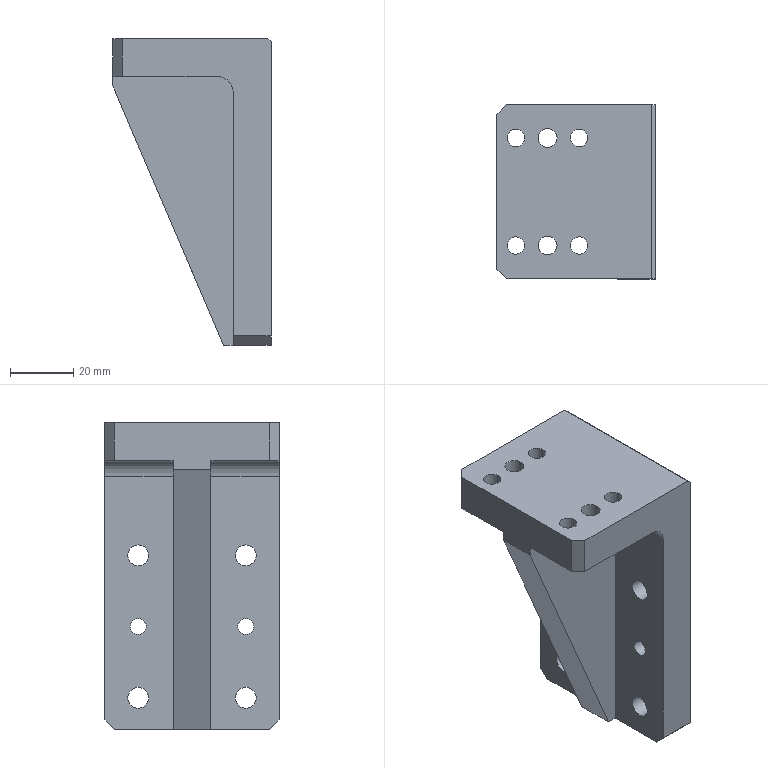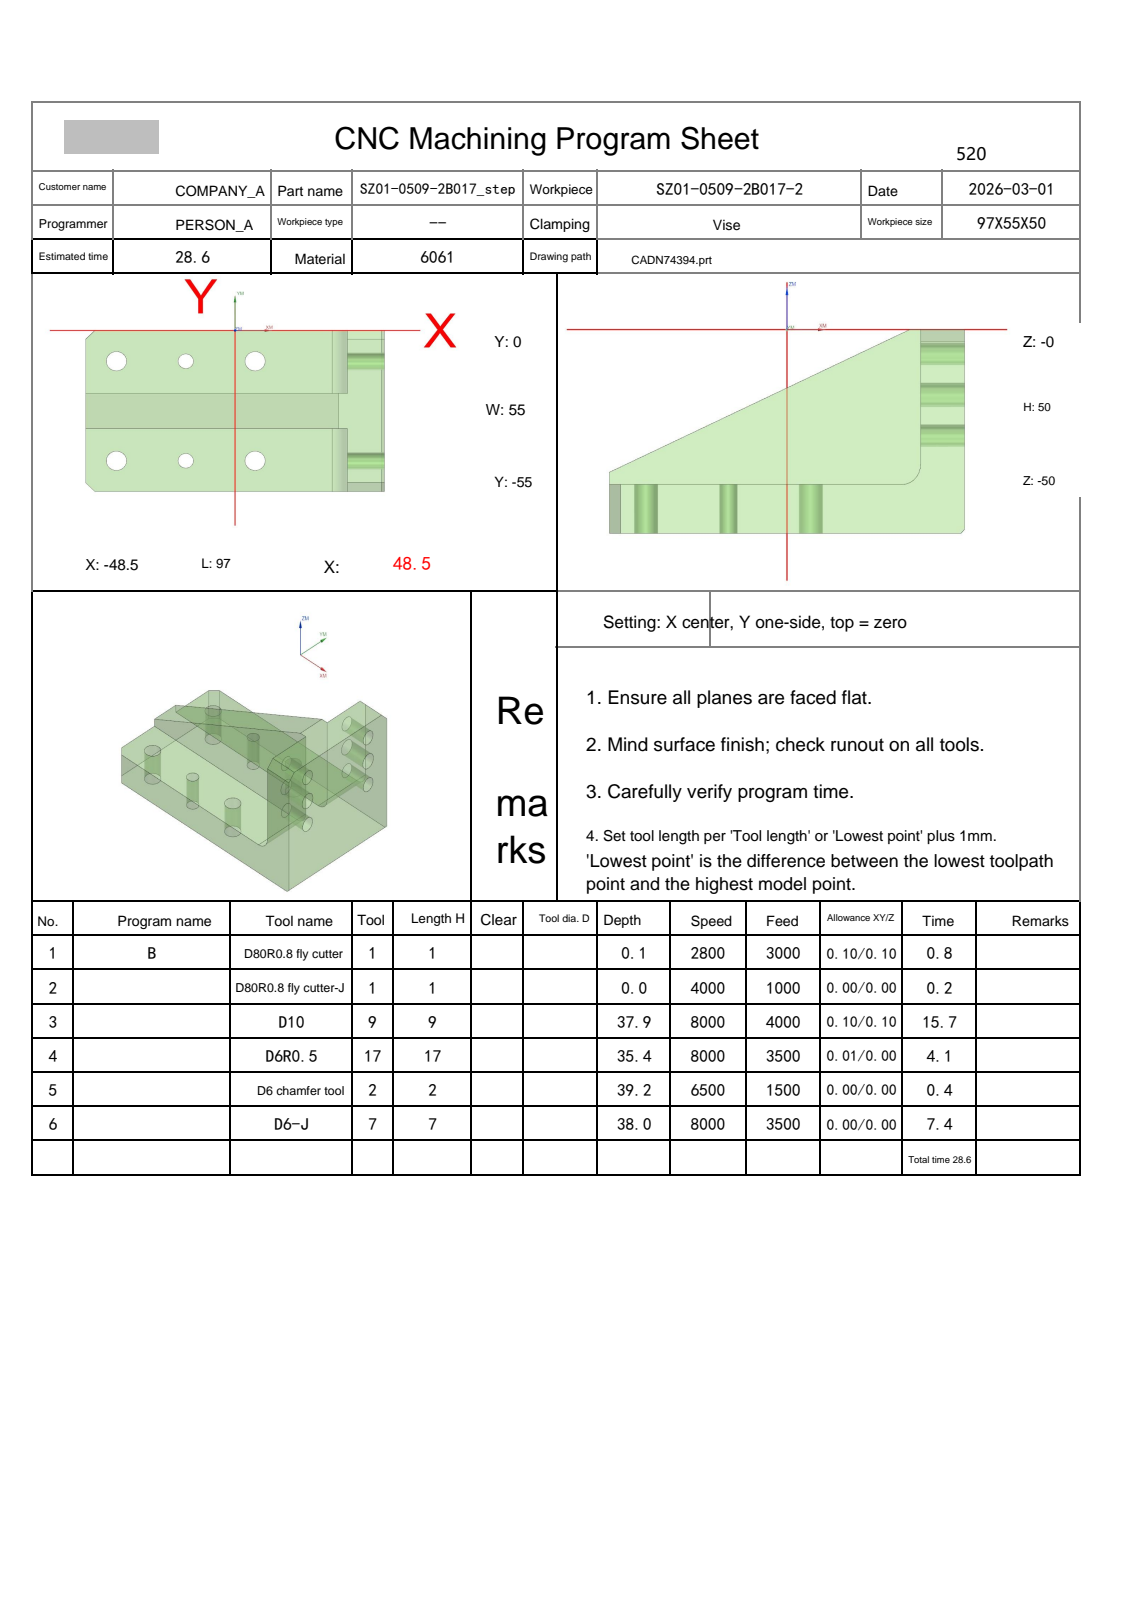NC program | NX | posted by the shop | part box 50 x 55 x 97 mm
Lines 1 to 109 of 18128:
%
O0001
(Machine time: 29.69 MIN)
(===Total Tool:5===)
(T1=D80R0.8 fly cutter D=80.  R=0.8  D-  H01 Z=0.    )
(T9=D10     D=10.  R=0.   D-  H09 Z=-37.9 )
(T17=D6R0.5 D=6.   R=0.5  D-  H17 Z=-35.45)
(T2=D6 chamfer tool   D=6.   R=0.   D-  H02 Z=-39.2 )
(T7=D6-J    D=6.   R=0.   D7  H07 Z=-38.  )
G80 G90 G17 G49 G40
G91 G28 Z0
M01
N1 T01 M06
(D80R0.8 fly cutter  D=80. R=0.8 H=01 ce=0.10 di=0.10)
G00 G90 G54 X-100.597 Y-27.5 M03 S2800
G43 H01 Z50.
M08
Z6.011
G01 Z4.011 F3000.
X-88.597
X88.597
X100.597
Z6.011
G00 X-100.597
Z5.522
G01 Z3.522
X-88.597
X88.597
X100.597
Z5.522
G00 X-100.597
Z5.033
G01 Z3.033
X-88.597
X88.597
X100.597
Z5.033
G00 X-100.597
Z4.544
G01 Z2.544
X-88.597
X88.597
X100.597
Z4.544
G00 Z50.
X-100.597
Z4.056
G01 Z2.056
X-88.597
X88.597
X100.597
Z4.056
G00 Z50.
X-100.597
Z3.567
G01 Z1.567
X-88.597
X88.597
X100.597
Z3.567
G00 Z50.
X-100.597
Z3.078
G01 Z1.078
X-88.597
X88.597
X100.597
Z3.078
G00 Z50.
X-100.597
Z2.589
G01 Z.589
X-88.597
X88.597
X100.597
Z2.589
G00 Z50.
X-100.597
Z2.1
G01 Z.1
X-88.597
X88.597
X100.597
Z2.1
G00 Z50.
G91 G28 Z0.0
M05
M09
G91 G28 Z0.0
M01
N2 T01 M06
(D80R0.8 fly cutter-J  D=80. R=0.8 H=01 ce=0.00 di=0.00)
G00 G90 G54 X-100.499 Y-27.5 M03 S4000
G43 H01 Z50.
M08
Z2.
G01 Z0.0 F1000.
X-88.499
X88.499
X100.499
Z2.
G00 Z50.
G91 G28 Z0.0
M05
M09
G91 G28 Z0.0
M01